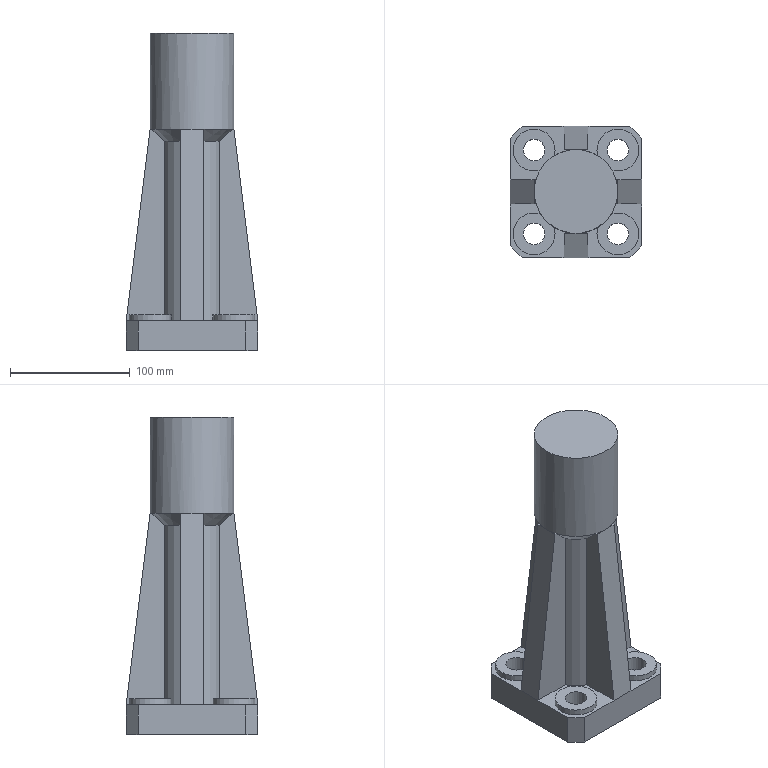Part | NX | features solid 2 | 1 solid | 55 faces | box 110 x 110 x 265 mm | volume 1177803 mm3 | plane 38 | cylinder 13 | cone 4 | commonest cylinder face diameters 18 x4 35 x4 50 x4 70 x1
STEP:
#1=CARTESIAN_POINT('',(935.,-402.087,-260.));
#2=VERTEX_POINT('',#1);
#3=CARTESIAN_POINT('',(935.,-402.087,-110.));
#4=VERTEX_POINT('',#3);
#5=CARTESIAN_POINT('',(935.,-402.087,-80.));
#6=DIRECTION('',(0.,0.,-1.));
#7=VECTOR('',#6,1000.);
#8=LINE('',#5,#7);
#9=EDGE_CURVE('',#2,#4,#8,.F.);
#10=ORIENTED_EDGE('',*,*,#9,.F.);
#11=CARTESIAN_POINT('',(922.087,-415.,-260.));
#12=VERTEX_POINT('',#11);
#13=CARTESIAN_POINT('',(945.,-425.,-260.));
#14=DIRECTION('',(0.,0.,1.));
#15=DIRECTION('',(1.,0.,0.));
#16=AXIS2_PLACEMENT_3D('',#13,#14,#15);
#17=CIRCLE('',#16,25.);
#18=EDGE_CURVE('',#12,#2,#17,.F.);
#19=ORIENTED_EDGE('',*,*,#18,.F.);
#20=CARTESIAN_POINT('',(922.087,-415.,-110.));
#21=VERTEX_POINT('',#20);
#22=CARTESIAN_POINT('',(922.087,-415.,-80.));
#23=DIRECTION('',(0.,0.,-1.));
#24=VECTOR('',#23,1000.);
#25=LINE('',#22,#24);
#26=EDGE_CURVE('',#12,#21,#25,.F.);
#27=ORIENTED_EDGE('',*,*,#26,.T.);
#28=CARTESIAN_POINT('',(945.,-425.,-110.));
#29=DIRECTION('',(0.,0.,1.));
#30=DIRECTION('',(1.,0.,0.));
#31=AXIS2_PLACEMENT_3D('',#28,#29,#30);
#32=CIRCLE('',#31,25.);
#33=EDGE_CURVE('',#21,#4,#32,.F.);
#34=ORIENTED_EDGE('',*,*,#33,.T.);
#35=EDGE_LOOP('',(#10,#19,#27,#34));
#36=FACE_BOUND('',#35,.T.);
#37=CARTESIAN_POINT('',(945.,-425.,-80.));
#38=DIRECTION('',(0.,0.,-1.));
#39=DIRECTION('',(-1.,0.,0.));
#40=AXIS2_PLACEMENT_3D('',#37,#38,#39);
#41=CYLINDRICAL_SURFACE('',#40,25.);
#42=ADVANCED_FACE('',(#36),#41,.T.);
#43=CARTESIAN_POINT('',(935.,-391.459,-100.));
#44=VERTEX_POINT('',#43);
#45=CARTESIAN_POINT('',(935.,-391.459,-100.));
#46=CARTESIAN_POINT('',(935.,-394.971,-103.366));
#47=CARTESIAN_POINT('',(935.,-398.501,-106.713));
#48=CARTESIAN_POINT('',(935.,-402.087,-110.));
#49=B_SPLINE_CURVE_WITH_KNOTS('',3,(#45,#46,#47,#48),.UNSPECIFIED.,.F.,.F.,(4,4),(0.01718,0.03177),.UNSPECIFIED.);
#50=EDGE_CURVE('',#4,#44,#49,.F.);
#51=ORIENTED_EDGE('',*,*,#50,.F.);
#52=ORIENTED_EDGE('',*,*,#33,.F.);
#53=CARTESIAN_POINT('',(911.459,-415.,-100.));
#54=VERTEX_POINT('',#53);
#55=CARTESIAN_POINT('',(911.459,-415.,-100.));
#56=CARTESIAN_POINT('',(914.971,-415.,-103.366));
#57=CARTESIAN_POINT('',(918.501,-415.,-106.713));
#58=CARTESIAN_POINT('',(922.087,-415.,-110.));
#59=B_SPLINE_CURVE_WITH_KNOTS('',3,(#55,#56,#57,#58),.UNSPECIFIED.,.F.,.F.,(4,4),(0.02378,0.03837),.UNSPECIFIED.);
#60=EDGE_CURVE('',#21,#54,#59,.F.);
#61=ORIENTED_EDGE('',*,*,#60,.T.);
#62=CARTESIAN_POINT('',(945.,-425.,-100.));
#63=DIRECTION('',(0.,0.,1.));
#64=DIRECTION('',(1.,0.,0.));
#65=AXIS2_PLACEMENT_3D('',#62,#63,#64);
#66=CIRCLE('',#65,35.);
#67=EDGE_CURVE('',#44,#54,#66,.T.);
#68=ORIENTED_EDGE('',*,*,#67,.F.);
#69=EDGE_LOOP('',(#51,#52,#61,#68));
#70=FACE_BOUND('',#69,.T.);
#71=CARTESIAN_POINT('',(945.,-425.,-100.));
#72=DIRECTION('',(0.,0.,1.));
#73=DIRECTION('',(1.,0.,0.));
#74=AXIS2_PLACEMENT_3D('',#71,#72,#73);
#75=CONICAL_SURFACE('',#74,35.,0.7854);
#76=ADVANCED_FACE('',(#70),#75,.T.);
#77=CARTESIAN_POINT('',(927.5,-390.,-260.));
#78=VERTEX_POINT('',#77);
#79=CARTESIAN_POINT('',(910.,-390.,-260.));
#80=DIRECTION('',(0.,0.,1.));
#81=DIRECTION('',(1.,0.,0.));
#82=AXIS2_PLACEMENT_3D('',#79,#80,#81);
#83=CIRCLE('',#82,17.5);
#84=EDGE_CURVE('',#78,#78,#83,.T.);
#85=ORIENTED_EDGE('',*,*,#84,.F.);
#86=EDGE_LOOP('',(#85));
#87=FACE_BOUND('',#86,.T.);
#88=CARTESIAN_POINT('',(900.,-370.,-260.));
#89=VERTEX_POINT('',#88);
#90=CARTESIAN_POINT('',(935.,-370.,-260.));
#91=VERTEX_POINT('',#90);
#92=CARTESIAN_POINT('',(890.,-370.,-260.));
#93=DIRECTION('',(1.,0.,0.));
#94=VECTOR('',#93,1000.);
#95=LINE('',#92,#94);
#96=EDGE_CURVE('',#89,#91,#95,.T.);
#97=ORIENTED_EDGE('',*,*,#96,.F.);
#98=CARTESIAN_POINT('',(890.,-380.,-260.));
#99=VERTEX_POINT('',#98);
#100=CARTESIAN_POINT('',(867.5,-402.5,-260.));
#101=DIRECTION('',(-0.7071,-0.7071,0.));
#102=VECTOR('',#101,1000.);
#103=LINE('',#100,#102);
#104=EDGE_CURVE('',#89,#99,#103,.T.);
#105=ORIENTED_EDGE('',*,*,#104,.T.);
#106=CARTESIAN_POINT('',(890.,-415.,-260.));
#107=VERTEX_POINT('',#106);
#108=CARTESIAN_POINT('',(890.,-425.,-260.));
#109=DIRECTION('',(0.,-1.,0.));
#110=VECTOR('',#109,1000.);
#111=LINE('',#108,#110);
#112=EDGE_CURVE('',#107,#99,#111,.F.);
#113=ORIENTED_EDGE('',*,*,#112,.F.);
#114=CARTESIAN_POINT('',(890.,-415.,-260.));
#115=DIRECTION('',(-1.,0.,0.));
#116=VECTOR('',#115,1000.);
#117=LINE('',#114,#116);
#118=EDGE_CURVE('',#12,#107,#117,.T.);
#119=ORIENTED_EDGE('',*,*,#118,.F.);
#120=ORIENTED_EDGE('',*,*,#18,.T.);
#121=CARTESIAN_POINT('',(935.,-425.,-260.));
#122=DIRECTION('',(0.,1.,0.));
#123=VECTOR('',#122,1000.);
#124=LINE('',#121,#123);
#125=EDGE_CURVE('',#2,#91,#124,.T.);
#126=ORIENTED_EDGE('',*,*,#125,.T.);
#127=EDGE_LOOP('',(#97,#105,#113,#119,#120,#126));
#128=FACE_BOUND('',#127,.T.);
#129=CARTESIAN_POINT('',(890.,-425.,-260.));
#130=DIRECTION('',(0.,0.,1.));
#131=DIRECTION('',(1.,0.,0.));
#132=AXIS2_PLACEMENT_3D('',#129,#130,#131);
#133=PLANE('',#132);
#134=ADVANCED_FACE('',(#87,#128),#133,.T.);
#135=CARTESIAN_POINT('',(922.087,-435.,-260.));
#136=VERTEX_POINT('',#135);
#137=CARTESIAN_POINT('',(922.087,-435.,-110.));
#138=VERTEX_POINT('',#137);
#139=CARTESIAN_POINT('',(922.087,-435.,-80.));
#140=DIRECTION('',(0.,0.,-1.));
#141=VECTOR('',#140,1000.);
#142=LINE('',#139,#141);
#143=EDGE_CURVE('',#136,#138,#142,.F.);
#144=ORIENTED_EDGE('',*,*,#143,.F.);
#145=CARTESIAN_POINT('',(935.,-447.913,-260.));
#146=VERTEX_POINT('',#145);
#147=CARTESIAN_POINT('',(945.,-425.,-260.));
#148=DIRECTION('',(0.,0.,1.));
#149=DIRECTION('',(1.,0.,0.));
#150=AXIS2_PLACEMENT_3D('',#147,#148,#149);
#151=CIRCLE('',#150,25.);
#152=EDGE_CURVE('',#146,#136,#151,.F.);
#153=ORIENTED_EDGE('',*,*,#152,.F.);
#154=CARTESIAN_POINT('',(935.,-447.913,-110.));
#155=VERTEX_POINT('',#154);
#156=CARTESIAN_POINT('',(935.,-447.913,-80.));
#157=DIRECTION('',(0.,0.,-1.));
#158=VECTOR('',#157,1000.);
#159=LINE('',#156,#158);
#160=EDGE_CURVE('',#146,#155,#159,.F.);
#161=ORIENTED_EDGE('',*,*,#160,.T.);
#162=CARTESIAN_POINT('',(945.,-425.,-110.));
#163=DIRECTION('',(0.,0.,1.));
#164=DIRECTION('',(1.,0.,0.));
#165=AXIS2_PLACEMENT_3D('',#162,#163,#164);
#166=CIRCLE('',#165,25.);
#167=EDGE_CURVE('',#155,#138,#166,.F.);
#168=ORIENTED_EDGE('',*,*,#167,.T.);
#169=EDGE_LOOP('',(#144,#153,#161,#168));
#170=FACE_BOUND('',#169,.T.);
#171=CARTESIAN_POINT('',(945.,-425.,-80.));
#172=DIRECTION('',(0.,0.,-1.));
#173=DIRECTION('',(-1.,0.,0.));
#174=AXIS2_PLACEMENT_3D('',#171,#172,#173);
#175=CYLINDRICAL_SURFACE('',#174,25.);
#176=ADVANCED_FACE('',(#170),#175,.T.);
#177=CARTESIAN_POINT('',(911.459,-435.,-100.));
#178=VERTEX_POINT('',#177);
#179=CARTESIAN_POINT('',(911.459,-435.,-100.));
#180=CARTESIAN_POINT('',(914.971,-435.,-103.366));
#181=CARTESIAN_POINT('',(918.501,-435.,-106.713));
#182=CARTESIAN_POINT('',(922.087,-435.,-110.));
#183=B_SPLINE_CURVE_WITH_KNOTS('',3,(#179,#180,#181,#182),.UNSPECIFIED.,.F.,.F.,(4,4),(0.02378,0.03837),.UNSPECIFIED.);
#184=EDGE_CURVE('',#138,#178,#183,.F.);
#185=ORIENTED_EDGE('',*,*,#184,.F.);
#186=ORIENTED_EDGE('',*,*,#167,.F.);
#187=CARTESIAN_POINT('',(935.,-458.541,-100.));
#188=VERTEX_POINT('',#187);
#189=CARTESIAN_POINT('',(935.,-458.541,-100.));
#190=CARTESIAN_POINT('',(935.,-455.029,-103.366));
#191=CARTESIAN_POINT('',(935.,-451.499,-106.713));
#192=CARTESIAN_POINT('',(935.,-447.913,-110.));
#193=B_SPLINE_CURVE_WITH_KNOTS('',3,(#189,#190,#191,#192),.UNSPECIFIED.,.F.,.F.,(4,4),(0.02378,0.03837),.UNSPECIFIED.);
#194=EDGE_CURVE('',#155,#188,#193,.F.);
#195=ORIENTED_EDGE('',*,*,#194,.T.);
#196=CARTESIAN_POINT('',(945.,-425.,-100.));
#197=DIRECTION('',(0.,0.,1.));
#198=DIRECTION('',(1.,0.,0.));
#199=AXIS2_PLACEMENT_3D('',#196,#197,#198);
#200=CIRCLE('',#199,35.);
#201=EDGE_CURVE('',#178,#188,#200,.T.);
#202=ORIENTED_EDGE('',*,*,#201,.F.);
#203=EDGE_LOOP('',(#185,#186,#195,#202));
#204=FACE_BOUND('',#203,.T.);
#205=CARTESIAN_POINT('',(945.,-425.,-100.));
#206=DIRECTION('',(0.,0.,1.));
#207=DIRECTION('',(1.,0.,0.));
#208=AXIS2_PLACEMENT_3D('',#205,#206,#207);
#209=CONICAL_SURFACE('',#208,35.,0.7854);
#210=ADVANCED_FACE('',(#204),#209,.T.);
#211=CARTESIAN_POINT('',(927.5,-460.,-260.));
#212=VERTEX_POINT('',#211);
#213=CARTESIAN_POINT('',(910.,-460.,-260.));
#214=DIRECTION('',(0.,0.,1.));
#215=DIRECTION('',(1.,0.,0.));
#216=AXIS2_PLACEMENT_3D('',#213,#214,#215);
#217=CIRCLE('',#216,17.5);
#218=EDGE_CURVE('',#212,#212,#217,.T.);
#219=ORIENTED_EDGE('',*,*,#218,.F.);
#220=EDGE_LOOP('',(#219));
#221=FACE_BOUND('',#220,.T.);
#222=CARTESIAN_POINT('',(890.,-470.,-260.));
#223=VERTEX_POINT('',#222);
#224=CARTESIAN_POINT('',(890.,-435.,-260.));
#225=VERTEX_POINT('',#224);
#226=CARTESIAN_POINT('',(890.,-425.,-260.));
#227=DIRECTION('',(0.,-1.,0.));
#228=VECTOR('',#227,1000.);
#229=LINE('',#226,#228);
#230=EDGE_CURVE('',#223,#225,#229,.F.);
#231=ORIENTED_EDGE('',*,*,#230,.F.);
#232=CARTESIAN_POINT('',(900.,-480.,-260.));
#233=VERTEX_POINT('',#232);
#234=CARTESIAN_POINT('',(867.5,-447.5,-260.));
#235=DIRECTION('',(-0.7071,0.7071,0.));
#236=VECTOR('',#235,1000.);
#237=LINE('',#234,#236);
#238=EDGE_CURVE('',#223,#233,#237,.F.);
#239=ORIENTED_EDGE('',*,*,#238,.T.);
#240=CARTESIAN_POINT('',(935.,-480.,-260.));
#241=VERTEX_POINT('',#240);
#242=CARTESIAN_POINT('',(890.,-480.,-260.));
#243=DIRECTION('',(1.,0.,0.));
#244=VECTOR('',#243,1000.);
#245=LINE('',#242,#244);
#246=EDGE_CURVE('',#233,#241,#245,.T.);
#247=ORIENTED_EDGE('',*,*,#246,.T.);
#248=CARTESIAN_POINT('',(935.,-425.,-260.));
#249=DIRECTION('',(0.,-1.,0.));
#250=VECTOR('',#249,1000.);
#251=LINE('',#248,#250);
#252=EDGE_CURVE('',#146,#241,#251,.T.);
#253=ORIENTED_EDGE('',*,*,#252,.F.);
#254=ORIENTED_EDGE('',*,*,#152,.T.);
#255=CARTESIAN_POINT('',(890.,-435.,-260.));
#256=DIRECTION('',(-1.,0.,0.));
#257=VECTOR('',#256,1000.);
#258=LINE('',#255,#257);
#259=EDGE_CURVE('',#136,#225,#258,.T.);
#260=ORIENTED_EDGE('',*,*,#259,.T.);
#261=EDGE_LOOP('',(#231,#239,#247,#253,#254,#260));
#262=FACE_BOUND('',#261,.T.);
#263=CARTESIAN_POINT('',(890.,-425.,-260.));
#264=DIRECTION('',(0.,0.,1.));
#265=DIRECTION('',(1.,0.,0.));
#266=AXIS2_PLACEMENT_3D('',#263,#264,#265);
#267=PLANE('',#266);
#268=ADVANCED_FACE('',(#221,#262),#267,.T.);
#269=CARTESIAN_POINT('',(955.,-402.087,-260.));
#270=VERTEX_POINT('',#269);
#271=CARTESIAN_POINT('',(967.913,-415.,-260.));
#272=VERTEX_POINT('',#271);
#273=CARTESIAN_POINT('',(945.,-425.,-260.));
#274=DIRECTION('',(0.,0.,1.));
#275=DIRECTION('',(1.,0.,0.));
#276=AXIS2_PLACEMENT_3D('',#273,#274,#275);
#277=CIRCLE('',#276,25.);
#278=EDGE_CURVE('',#270,#272,#277,.F.);
#279=ORIENTED_EDGE('',*,*,#278,.F.);
#280=CARTESIAN_POINT('',(955.,-402.087,-110.));
#281=VERTEX_POINT('',#280);
#282=CARTESIAN_POINT('',(955.,-402.087,-80.));
#283=DIRECTION('',(0.,0.,-1.));
#284=VECTOR('',#283,1000.);
#285=LINE('',#282,#284);
#286=EDGE_CURVE('',#270,#281,#285,.F.);
#287=ORIENTED_EDGE('',*,*,#286,.T.);
#288=CARTESIAN_POINT('',(967.913,-415.,-110.));
#289=VERTEX_POINT('',#288);
#290=CARTESIAN_POINT('',(945.,-425.,-110.));
#291=DIRECTION('',(0.,0.,1.));
#292=DIRECTION('',(1.,0.,0.));
#293=AXIS2_PLACEMENT_3D('',#290,#291,#292);
#294=CIRCLE('',#293,25.);
#295=EDGE_CURVE('',#281,#289,#294,.F.);
#296=ORIENTED_EDGE('',*,*,#295,.T.);
#297=CARTESIAN_POINT('',(967.913,-415.,-80.));
#298=DIRECTION('',(0.,0.,-1.));
#299=VECTOR('',#298,1000.);
#300=LINE('',#297,#299);
#301=EDGE_CURVE('',#272,#289,#300,.F.);
#302=ORIENTED_EDGE('',*,*,#301,.F.);
#303=EDGE_LOOP('',(#279,#287,#296,#302));
#304=FACE_BOUND('',#303,.T.);
#305=CARTESIAN_POINT('',(945.,-425.,-80.));
#306=DIRECTION('',(0.,0.,-1.));
#307=DIRECTION('',(-1.,0.,0.));
#308=AXIS2_PLACEMENT_3D('',#305,#306,#307);
#309=CYLINDRICAL_SURFACE('',#308,25.);
#310=ADVANCED_FACE('',(#304),#309,.T.);
#311=ORIENTED_EDGE('',*,*,#295,.F.);
#312=CARTESIAN_POINT('',(955.,-391.459,-100.));
#313=VERTEX_POINT('',#312);
#314=CARTESIAN_POINT('',(955.,-391.459,-100.));
#315=CARTESIAN_POINT('',(955.,-394.971,-103.366));
#316=CARTESIAN_POINT('',(955.,-398.501,-106.713));
#317=CARTESIAN_POINT('',(955.,-402.087,-110.));
#318=B_SPLINE_CURVE_WITH_KNOTS('',3,(#314,#315,#316,#317),.UNSPECIFIED.,.F.,.F.,(4,4),(0.01718,0.03177),.UNSPECIFIED.);
#319=EDGE_CURVE('',#281,#313,#318,.F.);
#320=ORIENTED_EDGE('',*,*,#319,.T.);
#321=CARTESIAN_POINT('',(978.541,-415.,-100.));
#322=VERTEX_POINT('',#321);
#323=CARTESIAN_POINT('',(945.,-425.,-100.));
#324=DIRECTION('',(0.,0.,1.));
#325=DIRECTION('',(1.,0.,0.));
#326=AXIS2_PLACEMENT_3D('',#323,#324,#325);
#327=CIRCLE('',#326,35.);
#328=EDGE_CURVE('',#322,#313,#327,.T.);
#329=ORIENTED_EDGE('',*,*,#328,.F.);
#330=CARTESIAN_POINT('',(978.541,-415.,-100.));
#331=CARTESIAN_POINT('',(975.029,-415.,-103.366));
#332=CARTESIAN_POINT('',(971.499,-415.,-106.713));
#333=CARTESIAN_POINT('',(967.913,-415.,-110.));
#334=B_SPLINE_CURVE_WITH_KNOTS('',3,(#330,#331,#332,#333),.UNSPECIFIED.,.F.,.F.,(4,4),(0.01718,0.03177),.UNSPECIFIED.);
#335=EDGE_CURVE('',#289,#322,#334,.F.);
#336=ORIENTED_EDGE('',*,*,#335,.F.);
#337=EDGE_LOOP('',(#311,#320,#329,#336));
#338=FACE_BOUND('',#337,.T.);
#339=CARTESIAN_POINT('',(945.,-425.,-100.));
#340=DIRECTION('',(0.,0.,1.));
#341=DIRECTION('',(1.,0.,0.));
#342=AXIS2_PLACEMENT_3D('',#339,#340,#341);
#343=CONICAL_SURFACE('',#342,35.,0.7854);
#344=ADVANCED_FACE('',(#338),#343,.T.);
#345=CARTESIAN_POINT('',(997.5,-390.,-260.));
#346=VERTEX_POINT('',#345);
#347=CARTESIAN_POINT('',(980.,-390.,-260.));
#348=DIRECTION('',(0.,0.,1.));
#349=DIRECTION('',(1.,0.,0.));
#350=AXIS2_PLACEMENT_3D('',#347,#348,#349);
#351=CIRCLE('',#350,17.5);
#352=EDGE_CURVE('',#346,#346,#351,.T.);
#353=ORIENTED_EDGE('',*,*,#352,.F.);
#354=EDGE_LOOP('',(#353));
#355=FACE_BOUND('',#354,.T.);
#356=CARTESIAN_POINT('',(1000.,-415.,-260.));
#357=VERTEX_POINT('',#356);
#358=CARTESIAN_POINT('',(1000.,-380.,-260.));
#359=VERTEX_POINT('',#358);
#360=CARTESIAN_POINT('',(1000.,-425.,-260.));
#361=DIRECTION('',(0.,1.,0.));
#362=VECTOR('',#361,1000.);
#363=LINE('',#360,#362);
#364=EDGE_CURVE('',#357,#359,#363,.T.);
#365=ORIENTED_EDGE('',*,*,#364,.T.);
#366=CARTESIAN_POINT('',(990.,-370.,-260.));
#367=VERTEX_POINT('',#366);
#368=CARTESIAN_POINT('',(967.5,-347.5,-260.));
#369=DIRECTION('',(0.7071,-0.7071,0.));
#370=VECTOR('',#369,1000.);
#371=LINE('',#368,#370);
#372=EDGE_CURVE('',#359,#367,#371,.F.);
#373=ORIENTED_EDGE('',*,*,#372,.T.);
#374=CARTESIAN_POINT('',(955.,-370.,-260.));
#375=VERTEX_POINT('',#374);
#376=CARTESIAN_POINT('',(890.,-370.,-260.));
#377=DIRECTION('',(1.,0.,0.));
#378=VECTOR('',#377,1000.);
#379=LINE('',#376,#378);
#380=EDGE_CURVE('',#375,#367,#379,.T.);
#381=ORIENTED_EDGE('',*,*,#380,.F.);
#382=CARTESIAN_POINT('',(955.,-425.,-260.));
#383=DIRECTION('',(0.,1.,0.));
#384=VECTOR('',#383,1000.);
#385=LINE('',#382,#384);
#386=EDGE_CURVE('',#270,#375,#385,.T.);
#387=ORIENTED_EDGE('',*,*,#386,.F.);
#388=ORIENTED_EDGE('',*,*,#278,.T.);
#389=CARTESIAN_POINT('',(890.,-415.,-260.));
#390=DIRECTION('',(1.,0.,0.));
#391=VECTOR('',#390,1000.);
#392=LINE('',#389,#391);
#393=EDGE_CURVE('',#272,#357,#392,.T.);
#394=ORIENTED_EDGE('',*,*,#393,.T.);
#395=EDGE_LOOP('',(#365,#373,#381,#387,#388,#394));
#396=FACE_BOUND('',#395,.T.);
#397=CARTESIAN_POINT('',(890.,-425.,-260.));
#398=DIRECTION('',(0.,0.,1.));
#399=DIRECTION('',(1.,0.,0.));
#400=AXIS2_PLACEMENT_3D('',#397,#398,#399);
#401=PLANE('',#400);
#402=ADVANCED_FACE('',(#355,#396),#401,.T.);
#403=CARTESIAN_POINT('',(967.913,-435.,-260.));
#404=VERTEX_POINT('',#403);
#405=CARTESIAN_POINT('',(955.,-447.913,-260.));
#406=VERTEX_POINT('',#405);
#407=CARTESIAN_POINT('',(945.,-425.,-260.));
#408=DIRECTION('',(0.,0.,1.));
#409=DIRECTION('',(1.,0.,0.));
#410=AXIS2_PLACEMENT_3D('',#407,#408,#409);
#411=CIRCLE('',#410,25.);
#412=EDGE_CURVE('',#404,#406,#411,.F.);
#413=ORIENTED_EDGE('',*,*,#412,.F.);
#414=CARTESIAN_POINT('',(967.913,-435.,-110.));
#415=VERTEX_POINT('',#414);
#416=CARTESIAN_POINT('',(967.913,-435.,-80.));
#417=DIRECTION('',(0.,0.,-1.));
#418=VECTOR('',#417,1000.);
#419=LINE('',#416,#418);
#420=EDGE_CURVE('',#404,#415,#419,.F.);
#421=ORIENTED_EDGE('',*,*,#420,.T.);
#422=CARTESIAN_POINT('',(955.,-447.913,-110.));
#423=VERTEX_POINT('',#422);
#424=CARTESIAN_POINT('',(945.,-425.,-110.));
#425=DIRECTION('',(0.,0.,1.));
#426=DIRECTION('',(1.,0.,0.));
#427=AXIS2_PLACEMENT_3D('',#424,#425,#426);
#428=CIRCLE('',#427,25.);
#429=EDGE_CURVE('',#415,#423,#428,.F.);
#430=ORIENTED_EDGE('',*,*,#429,.T.);
#431=CARTESIAN_POINT('',(955.,-447.913,-80.));
#432=DIRECTION('',(0.,0.,-1.));
#433=VECTOR('',#432,1000.);
#434=LINE('',#431,#433);
#435=EDGE_CURVE('',#406,#423,#434,.F.);
#436=ORIENTED_EDGE('',*,*,#435,.F.);
#437=EDGE_LOOP('',(#413,#421,#430,#436));
#438=FACE_BOUND('',#437,.T.);
#439=CARTESIAN_POINT('',(945.,-425.,-80.));
#440=DIRECTION('',(0.,0.,-1.));
#441=DIRECTION('',(-1.,0.,0.));
#442=AXIS2_PLACEMENT_3D('',#439,#440,#441);
#443=CYLINDRICAL_SURFACE('',#442,25.);
#444=ADVANCED_FACE('',(#438),#443,.T.);
#445=ORIENTED_EDGE('',*,*,#429,.F.);
#446=CARTESIAN_POINT('',(978.541,-435.,-100.));
#447=VERTEX_POINT('',#446);
#448=CARTESIAN_POINT('',(978.541,-435.,-100.));
#449=CARTESIAN_POINT('',(975.029,-435.,-103.366));
#450=CARTESIAN_POINT('',(971.499,-435.,-106.713));
#451=CARTESIAN_POINT('',(967.913,-435.,-110.));
#452=B_SPLINE_CURVE_WITH_KNOTS('',3,(#448,#449,#450,#451),.UNSPECIFIED.,.F.,.F.,(4,4),(0.01718,0.03177),.UNSPECIFIED.);
#453=EDGE_CURVE('',#415,#447,#452,.F.);
#454=ORIENTED_EDGE('',*,*,#453,.T.);
#455=CARTESIAN_POINT('',(955.,-458.541,-100.));
#456=VERTEX_POINT('',#455);
#457=CARTESIAN_POINT('',(945.,-425.,-100.));
#458=DIRECTION('',(0.,0.,1.));
#459=DIRECTION('',(1.,0.,0.));
#460=AXIS2_PLACEMENT_3D('',#457,#458,#459);
#461=CIRCLE('',#460,35.);
#462=EDGE_CURVE('',#456,#447,#461,.T.);
#463=ORIENTED_EDGE('',*,*,#462,.F.);
#464=CARTESIAN_POINT('',(955.,-458.541,-100.));
#465=CARTESIAN_POINT('',(955.,-455.029,-103.366));
#466=CARTESIAN_POINT('',(955.,-451.499,-106.713));
#467=CARTESIAN_POINT('',(955.,-447.913,-110.));
#468=B_SPLINE_CURVE_WITH_KNOTS('',3,(#464,#465,#466,#467),.UNSPECIFIED.,.F.,.F.,(4,4),(0.02378,0.03837),.UNSPECIFIED.);
#469=EDGE_CURVE('',#423,#456,#468,.F.);
#470=ORIENTED_EDGE('',*,*,#469,.F.);
#471=EDGE_LOOP('',(#445,#454,#463,#470));
#472=FACE_BOUND('',#471,.T.);
#473=CARTESIAN_POINT('',(945.,-425.,-100.));
#474=DIRECTION('',(0.,0.,1.));
#475=DIRECTION('',(1.,0.,0.));
#476=AXIS2_PLACEMENT_3D('',#473,#474,#475);
#477=CONICAL_SURFACE('',#476,35.,0.7854);
#478=ADVANCED_FACE('',(#472),#477,.T.);
#479=CARTESIAN_POINT('',(997.5,-460.,-260.));
#480=VERTEX_POINT('',#479);
#481=CARTESIAN_POINT('',(980.,-460.,-260.));
#482=DIRECTION('',(0.,0.,1.));
#483=DIRECTION('',(1.,0.,0.));
#484=AXIS2_PLACEMENT_3D('',#481,#482,#483);
#485=CIRCLE('',#484,17.5);
#486=EDGE_CURVE('',#480,#480,#485,.T.);
#487=ORIENTED_EDGE('',*,*,#486,.F.);
#488=EDGE_LOOP('',(#487));
#489=FACE_BOUND('',#488,.T.);
#490=CARTESIAN_POINT('',(955.,-480.,-260.));
#491=VERTEX_POINT('',#490);
#492=CARTESIAN_POINT('',(990.,-480.,-260.));
#493=VERTEX_POINT('',#492);
#494=CARTESIAN_POINT('',(890.,-480.,-260.));
#495=DIRECTION('',(1.,0.,0.));
#496=VECTOR('',#495,1000.);
#497=LINE('',#494,#496);
#498=EDGE_CURVE('',#491,#493,#497,.T.);
#499=ORIENTED_EDGE('',*,*,#498,.T.);
#500=CARTESIAN_POINT('',(1000.,-470.,-260.));
#501=VERTEX_POINT('',#500);
#502=CARTESIAN_POINT('',(967.5,-502.5,-260.));
#503=DIRECTION('',(0.7071,0.7071,0.));
#504=VECTOR('',#503,1000.);
#505=LINE('',#502,#504);
#506=EDGE_CURVE('',#493,#501,#505,.T.);
#507=ORIENTED_EDGE('',*,*,#506,.T.);
#508=CARTESIAN_POINT('',(1000.,-435.,-260.));
#509=VERTEX_POINT('',#508);
#510=CARTESIAN_POINT('',(1000.,-425.,-260.));
#511=DIRECTION('',(0.,1.,0.));
#512=VECTOR('',#511,1000.);
#513=LINE('',#510,#512);
#514=EDGE_CURVE('',#501,#509,#513,.T.);
#515=ORIENTED_EDGE('',*,*,#514,.T.);
#516=CARTESIAN_POINT('',(890.,-435.,-260.));
#517=DIRECTION('',(1.,0.,0.));
#518=VECTOR('',#517,1000.);
#519=LINE('',#516,#518);
#520=EDGE_CURVE('',#404,#509,#519,.T.);
#521=ORIENTED_EDGE('',*,*,#520,.F.);
#522=ORIENTED_EDGE('',*,*,#412,.T.);
#523=CARTESIAN_POINT('',(955.,-425.,-260.));
#524=DIRECTION('',(0.,-1.,0.));
#525=VECTOR('',#524,1000.);
#526=LINE('',#523,#525);
#527=EDGE_CURVE('',#406,#491,#526,.T.);
#528=ORIENTED_EDGE('',*,*,#527,.T.);
#529=EDGE_LOOP('',(#499,#507,#515,#521,#522,#528));
#530=FACE_BOUND('',#529,.T.);
#531=CARTESIAN_POINT('',(890.,-425.,-260.));
#532=DIRECTION('',(0.,0.,1.));
#533=DIRECTION('',(1.,0.,0.));
#534=AXIS2_PLACEMENT_3D('',#531,#532,#533);
#535=PLANE('',#534);
#536=ADVANCED_FACE('',(#489,#530),#535,.T.);
#537=CARTESIAN_POINT('',(945.,-460.,-100.));
#538=VERTEX_POINT('',#537);
#539=CARTESIAN_POINT('',(945.,-425.,-100.));
#540=DIRECTION('',(0.,0.,1.));
#541=DIRECTION('',(1.,0.,0.));
#542=AXIS2_PLACEMENT_3D('',#539,#540,#541);
#543=CIRCLE('',#542,35.);
#544=EDGE_CURVE('',#188,#538,#543,.T.);
#545=ORIENTED_EDGE('',*,*,#544,.T.);
#546=CARTESIAN_POINT('',(945.,-425.,-100.));
#547=DIRECTION('',(0.,0.,1.));
#548=DIRECTION('',(1.,0.,0.));
#549=AXIS2_PLACEMENT_3D('',#546,#547,#548);
#550=CIRCLE('',#549,35.);
#551=EDGE_CURVE('',#538,#456,#550,.T.);
#552=ORIENTED_EDGE('',*,*,#551,.T.);
#553=ORIENTED_EDGE('',*,*,#462,.T.);
#554=CARTESIAN_POINT('',(980.,-425.,-100.));
#555=VERTEX_POINT('',#554);
#556=CARTESIAN_POINT('',(945.,-425.,-100.));
#557=DIRECTION('',(0.,0.,1.));
#558=DIRECTION('',(1.,0.,0.));
#559=AXIS2_PLACEMENT_3D('',#556,#557,#558);
#560=CIRCLE('',#559,35.);
#561=EDGE_CURVE('',#447,#555,#560,.T.);
#562=ORIENTED_EDGE('',*,*,#561,.T.);
#563=CARTESIAN_POINT('',(945.,-425.,-100.));
#564=DIRECTION('',(0.,0.,1.));
#565=DIRECTION('',(1.,0.,0.));
#566=AXIS2_PLACEMENT_3D('',#563,#564,#565);
#567=CIRCLE('',#566,35.);
#568=EDGE_CURVE('',#555,#322,#567,.T.);
#569=ORIENTED_EDGE('',*,*,#568,.T.);
#570=ORIENTED_EDGE('',*,*,#328,.T.);
#571=CARTESIAN_POINT('',(945.,-390.,-100.));
#572=VERTEX_POINT('',#571);
#573=CARTESIAN_POINT('',(945.,-425.,-100.));
#574=DIRECTION('',(0.,0.,1.));
#575=DIRECTION('',(1.,0.,0.));
#576=AXIS2_PLACEMENT_3D('',#573,#574,#575);
#577=CIRCLE('',#576,35.);
#578=EDGE_CURVE('',#313,#572,#577,.T.);
#579=ORIENTED_EDGE('',*,*,#578,.T.);
#580=CARTESIAN_POINT('',(945.,-425.,-100.));
#581=DIRECTION('',(0.,0.,1.));
#582=DIRECTION('',(1.,0.,0.));
#583=AXIS2_PLACEMENT_3D('',#580,#581,#582);
#584=CIRCLE('',#583,35.);
#585=EDGE_CURVE('',#572,#44,#584,.T.);
#586=ORIENTED_EDGE('',*,*,#585,.T.);
#587=ORIENTED_EDGE('',*,*,#67,.T.);
#588=CARTESIAN_POINT('',(910.,-425.,-100.));
#589=VERTEX_POINT('',#588);
#590=CARTESIAN_POINT('',(945.,-425.,-100.));
#591=DIRECTION('',(0.,0.,1.));
#592=DIRECTION('',(1.,0.,0.));
#593=AXIS2_PLACEMENT_3D('',#590,#591,#592);
#594=CIRCLE('',#593,35.);
#595=EDGE_CURVE('',#54,#589,#594,.T.);
#596=ORIENTED_EDGE('',*,*,#595,.T.);
#597=CARTESIAN_POINT('',(945.,-425.,-100.));
#598=DIRECTION('',(0.,0.,1.));
#599=DIRECTION('',(1.,0.,0.));
#600=AXIS2_PLACEMENT_3D('',#597,#598,#599);
#601=CIRCLE('',#600,35.);
#602=EDGE_CURVE('',#589,#178,#601,.T.);
#603=ORIENTED_EDGE('',*,*,#602,.T.);
#604=ORIENTED_EDGE('',*,*,#201,.T.);
#605=EDGE_LOOP('',(#545,#552,#553,#562,#569,#570,#579,#586,#587,#596,#603,#604));
#606=FACE_BOUND('',#605,.T.);
#607=CARTESIAN_POINT('',(980.,-425.,-20.));
#608=VERTEX_POINT('',#607);
#609=CARTESIAN_POINT('',(945.,-425.,-20.));
#610=DIRECTION('',(0.,0.,-1.));
#611=DIRECTION('',(1.,0.,0.));
#612=AXIS2_PLACEMENT_3D('',#609,#610,#611);
#613=CIRCLE('',#612,35.);
#614=EDGE_CURVE('',#608,#608,#613,.F.);
#615=ORIENTED_EDGE('',*,*,#614,.F.);
#616=EDGE_LOOP('',(#615));
#617=FACE_BOUND('',#616,.T.);
#618=CARTESIAN_POINT('',(945.,-425.,-140.));
#619=DIRECTION('',(0.,0.,1.));
#620=DIRECTION('',(1.,0.,0.));
#621=AXIS2_PLACEMENT_3D('',#618,#619,#620);
#622=CYLINDRICAL_SURFACE('',#621,35.);
#623=ADVANCED_FACE('',(#606,#617),#622,.T.);
#624=ORIENTED_EDGE('',*,*,#614,.T.);
#625=EDGE_LOOP('',(#624));
#626=FACE_BOUND('',#625,.T.);
#627=CARTESIAN_POINT('',(945.,-425.,-20.));
#628=DIRECTION('',(0.,0.,1.));
#629=DIRECTION('',(1.,0.,0.));
#630=AXIS2_PLACEMENT_3D('',#627,#628,#629);
#631=PLANE('',#630);
#632=ADVANCED_FACE('',(#626),#631,.T.);
#633=CARTESIAN_POINT('',(1000.,-470.,-285.));
#634=VERTEX_POINT('',#633);
#635=CARTESIAN_POINT('',(1000.,-380.,-285.));
#636=VERTEX_POINT('',#635);
#637=CARTESIAN_POINT('',(1000.,-425.,-285.));
#638=DIRECTION('',(0.,-1.,0.));
#639=VECTOR('',#638,1000.);
#640=LINE('',#637,#639);
#641=EDGE_CURVE('',#634,#636,#640,.F.);
#642=ORIENTED_EDGE('',*,*,#641,.T.);
#643=CARTESIAN_POINT('',(1000.,-380.,-265.));
#644=DIRECTION('',(0.,0.,1.));
#645=VECTOR('',#644,1000.);
#646=LINE('',#643,#645);
#647=EDGE_CURVE('',#636,#359,#646,.T.);
#648=ORIENTED_EDGE('',*,*,#647,.T.);
#649=ORIENTED_EDGE('',*,*,#364,.F.);
#650=CARTESIAN_POINT('',(1000.,-425.,-260.));
#651=DIRECTION('',(0.,1.,0.));
#652=VECTOR('',#651,1000.);
#653=LINE('',#650,#652);
#654=EDGE_CURVE('',#357,#509,#653,.F.);
#655=ORIENTED_EDGE('',*,*,#654,.T.);
#656=ORIENTED_EDGE('',*,*,#514,.F.);
#657=CARTESIAN_POINT('',(1000.,-470.,-295.));
#658=DIRECTION('',(0.,0.,-1.));
#659=VECTOR('',#658,1000.);
#660=LINE('',#657,#659);
#661=EDGE_CURVE('',#501,#634,#660,.T.);
#662=ORIENTED_EDGE('',*,*,#661,.T.);
#663=EDGE_LOOP('',(#642,#648,#649,#655,#656,#662));
#664=FACE_BOUND('',#663,.T.);
#665=CARTESIAN_POINT('',(1000.,-425.,-265.));
#666=DIRECTION('',(1.,0.,0.));
#667=DIRECTION('',(0.,0.,-1.));
#668=AXIS2_PLACEMENT_3D('',#665,#666,#667);
#669=PLANE('',#668);
#670=ADVANCED_FACE('',(#664),#669,.T.);
#671=CARTESIAN_POINT('',(919.,-390.,-285.));
#672=VERTEX_POINT('',#671);
#673=CARTESIAN_POINT('',(910.,-390.,-285.));
#674=DIRECTION('',(0.,0.,1.));
#675=DIRECTION('',(1.,0.,0.));
#676=AXIS2_PLACEMENT_3D('',#673,#674,#675);
#677=CIRCLE('',#676,9.);
#678=EDGE_CURVE('',#672,#672,#677,.F.);
#679=ORIENTED_EDGE('',*,*,#678,.F.);
#680=EDGE_LOOP('',(#679));
#681=FACE_BOUND('',#680,.T.);
#682=CARTESIAN_POINT('',(989.,-390.,-285.));
#683=VERTEX_POINT('',#682);
#684=CARTESIAN_POINT('',(980.,-390.,-285.));
#685=DIRECTION('',(0.,0.,1.));
#686=DIRECTION('',(1.,0.,0.));
#687=AXIS2_PLACEMENT_3D('',#684,#685,#686);
#688=CIRCLE('',#687,9.);
#689=EDGE_CURVE('',#683,#683,#688,.F.);
#690=ORIENTED_EDGE('',*,*,#689,.F.);
#691=EDGE_LOOP('',(#690));
#692=FACE_BOUND('',#691,.T.);
#693=CARTESIAN_POINT('',(919.,-460.,-285.));
#694=VERTEX_POINT('',#693);
#695=CARTESIAN_POINT('',(910.,-460.,-285.));
#696=DIRECTION('',(0.,0.,1.));
#697=DIRECTION('',(1.,0.,0.));
#698=AXIS2_PLACEMENT_3D('',#695,#696,#697);
#699=CIRCLE('',#698,9.);
#700=EDGE_CURVE('',#694,#694,#699,.F.);
#701=ORIENTED_EDGE('',*,*,#700,.F.);
#702=EDGE_LOOP('',(#701));
#703=FACE_BOUND('',#702,.T.);
#704=CARTESIAN_POINT('',(989.,-460.,-285.));
#705=VERTEX_POINT('',#704);
#706=CARTESIAN_POINT('',(980.,-460.,-285.));
#707=DIRECTION('',(0.,0.,1.));
#708=DIRECTION('',(1.,0.,0.));
#709=AXIS2_PLACEMENT_3D('',#706,#707,#708);
#710=CIRCLE('',#709,9.);
#711=EDGE_CURVE('',#705,#705,#710,.F.);
#712=ORIENTED_EDGE('',*,*,#711,.F.);
#713=EDGE_LOOP('',(#712));
#714=FACE_BOUND('',#713,.T.);
#715=CARTESIAN_POINT('',(890.,-470.,-285.));
#716=VERTEX_POINT('',#715);
#717=CARTESIAN_POINT('',(890.,-380.,-285.));
#718=VERTEX_POINT('',#717);
#719=CARTESIAN_POINT('',(890.,-425.,-285.));
#720=DIRECTION('',(0.,1.,0.));
#721=VECTOR('',#720,1000.);
#722=LINE('',#719,#721);
#723=EDGE_CURVE('',#716,#718,#722,.T.);
#724=ORIENTED_EDGE('',*,*,#723,.T.);
#725=CARTESIAN_POINT('',(900.,-370.,-285.));
#726=VERTEX_POINT('',#725);
#727=CARTESIAN_POINT('',(867.5,-402.5,-285.));
#728=DIRECTION('',(-0.7071,-0.7071,0.));
#729=VECTOR('',#728,1000.);
#730=LINE('',#727,#729);
#731=EDGE_CURVE('',#718,#726,#730,.F.);
#732=ORIENTED_EDGE('',*,*,#731,.T.);
#733=CARTESIAN_POINT('',(990.,-370.,-285.));
#734=VERTEX_POINT('',#733);
#735=CARTESIAN_POINT('',(890.,-370.,-285.));
#736=DIRECTION('',(-1.,0.,0.));
#737=VECTOR('',#736,1000.);
#738=LINE('',#735,#737);
#739=EDGE_CURVE('',#726,#734,#738,.F.);
#740=ORIENTED_EDGE('',*,*,#739,.T.);
#741=CARTESIAN_POINT('',(967.5,-347.5,-285.));
#742=DIRECTION('',(0.7071,-0.7071,0.));
#743=VECTOR('',#742,1000.);
#744=LINE('',#741,#743);
#745=EDGE_CURVE('',#734,#636,#744,.T.);
#746=ORIENTED_EDGE('',*,*,#745,.T.);
#747=ORIENTED_EDGE('',*,*,#641,.F.);
#748=CARTESIAN_POINT('',(990.,-480.,-285.));
#749=VERTEX_POINT('',#748);
#750=CARTESIAN_POINT('',(967.5,-502.5,-285.));
#751=DIRECTION('',(0.7071,0.7071,0.));
#752=VECTOR('',#751,1000.);
#753=LINE('',#750,#752);
#754=EDGE_CURVE('',#634,#749,#753,.F.);
#755=ORIENTED_EDGE('',*,*,#754,.T.);
#756=CARTESIAN_POINT('',(900.,-480.,-285.));
#757=VERTEX_POINT('',#756);
#758=CARTESIAN_POINT('',(890.,-480.,-285.));
#759=DIRECTION('',(-1.,0.,0.));
#760=VECTOR('',#759,1000.);
#761=LINE('',#758,#760);
#762=EDGE_CURVE('',#757,#749,#761,.F.);
#763=ORIENTED_EDGE('',*,*,#762,.F.);
#764=CARTESIAN_POINT('',(867.5,-447.5,-285.));
#765=DIRECTION('',(-0.7071,0.7071,0.));
#766=VECTOR('',#765,1000.);
#767=LINE('',#764,#766);
#768=EDGE_CURVE('',#757,#716,#767,.T.);
#769=ORIENTED_EDGE('',*,*,#768,.T.);
#770=EDGE_LOOP('',(#724,#732,#740,#746,#747,#755,#763,#769));
#771=FACE_BOUND('',#770,.T.);
#772=CARTESIAN_POINT('',(890.,-425.,-285.));
#773=DIRECTION('',(0.,0.,1.));
#774=DIRECTION('',(1.,0.,0.));
#775=AXIS2_PLACEMENT_3D('',#772,#773,#774);
#776=PLANE('',#775);
#777=ADVANCED_FACE('',(#681,#692,#703,#714,#771),#776,.F.);
#778=ORIENTED_EDGE('',*,*,#112,.T.);
#779=CARTESIAN_POINT('',(890.,-380.,-265.));
#780=DIRECTION('',(0.,0.,1.));
#781=VECTOR('',#780,1000.);
#782=LINE('',#779,#781);
#783=EDGE_CURVE('',#99,#718,#782,.F.);
#784=ORIENTED_EDGE('',*,*,#783,.T.);
#785=ORIENTED_EDGE('',*,*,#723,.F.);
#786=CARTESIAN_POINT('',(890.,-470.,-270.));
#787=DIRECTION('',(0.,0.,-1.));
#788=VECTOR('',#787,1000.);
#789=LINE('',#786,#788);
#790=EDGE_CURVE('',#716,#223,#789,.F.);
#791=ORIENTED_EDGE('',*,*,#790,.T.);
#792=ORIENTED_EDGE('',*,*,#230,.T.);
#793=CARTESIAN_POINT('',(890.,-425.,-260.));
#794=DIRECTION('',(0.,-1.,0.));
#795=VECTOR('',#794,1000.);
#796=LINE('',#793,#795);
#797=EDGE_CURVE('',#225,#107,#796,.F.);
#798=ORIENTED_EDGE('',*,*,#797,.T.);
#799=EDGE_LOOP('',(#778,#784,#785,#791,#792,#798));
#800=FACE_BOUND('',#799,.T.);
#801=CARTESIAN_POINT('',(890.,-425.,-265.));
#802=DIRECTION('',(1.,0.,0.));
#803=DIRECTION('',(0.,0.,-1.));
#804=AXIS2_PLACEMENT_3D('',#801,#802,#803);
#805=PLANE('',#804);
#806=ADVANCED_FACE('',(#800),#805,.F.);
#807=ORIENTED_EDGE('',*,*,#739,.F.);
#808=CARTESIAN_POINT('',(900.,-370.,-265.));
#809=DIRECTION('',(0.,0.,1.));
#810=VECTOR('',#809,1000.);
#811=LINE('',#808,#810);
#812=EDGE_CURVE('',#726,#89,#811,.T.);
#813=ORIENTED_EDGE('',*,*,#812,.T.);
#814=ORIENTED_EDGE('',*,*,#96,.T.);
#815=CARTESIAN_POINT('',(945.,-370.,-260.));
#816=DIRECTION('',(-1.,0.,0.));
#817=VECTOR('',#816,1000.);
#818=LINE('',#815,#817);
#819=EDGE_CURVE('',#91,#375,#818,.F.);
#820=ORIENTED_EDGE('',*,*,#819,.T.);
#821=ORIENTED_EDGE('',*,*,#380,.T.);
#822=CARTESIAN_POINT('',(990.,-370.,-265.));
#823=DIRECTION('',(0.,0.,-1.));
#824=VECTOR('',#823,1000.);
#825=LINE('',#822,#824);
#826=EDGE_CURVE('',#367,#734,#825,.T.);
#827=ORIENTED_EDGE('',*,*,#826,.T.);
#828=EDGE_LOOP('',(#807,#813,#814,#820,#821,#827));
#829=FACE_BOUND('',#828,.T.);
#830=CARTESIAN_POINT('',(890.,-370.,-265.));
#831=DIRECTION('',(0.,1.,0.));
#832=DIRECTION('',(0.,0.,1.));
#833=AXIS2_PLACEMENT_3D('',#830,#831,#832);
#834=PLANE('',#833);
#835=ADVANCED_FACE('',(#829),#834,.T.);
#836=ORIENTED_EDGE('',*,*,#246,.F.);
#837=CARTESIAN_POINT('',(900.,-480.,-295.));
#838=DIRECTION('',(0.,0.,-1.));
#839=VECTOR('',#838,1000.);
#840=LINE('',#837,#839);
#841=EDGE_CURVE('',#233,#757,#840,.T.);
#842=ORIENTED_EDGE('',*,*,#841,.T.);
#843=ORIENTED_EDGE('',*,*,#762,.T.);
#844=CARTESIAN_POINT('',(990.,-480.,-270.));
#845=DIRECTION('',(0.,0.,1.));
#846=VECTOR('',#845,1000.);
#847=LINE('',#844,#846);
#848=EDGE_CURVE('',#749,#493,#847,.T.);
#849=ORIENTED_EDGE('',*,*,#848,.T.);
#850=ORIENTED_EDGE('',*,*,#498,.F.);
#851=CARTESIAN_POINT('',(945.,-480.,-260.));
#852=DIRECTION('',(1.,0.,0.));
#853=VECTOR('',#852,1000.);
#854=LINE('',#851,#853);
#855=EDGE_CURVE('',#491,#241,#854,.F.);
#856=ORIENTED_EDGE('',*,*,#855,.T.);
#857=EDGE_LOOP('',(#836,#842,#843,#849,#850,#856));
#858=FACE_BOUND('',#857,.T.);
#859=CARTESIAN_POINT('',(890.,-480.,-265.));
#860=DIRECTION('',(0.,1.,0.));
#861=DIRECTION('',(0.,0.,1.));
#862=AXIS2_PLACEMENT_3D('',#859,#860,#861);
#863=PLANE('',#862);
#864=ADVANCED_FACE('',(#858),#863,.F.);
#865=CARTESIAN_POINT('',(955.,-460.,-100.));
#866=VERTEX_POINT('',#865);
#867=CARTESIAN_POINT('',(955.,-450.,-100.));
#868=DIRECTION('',(0.,-1.,0.));
#869=VECTOR('',#868,1000.);
#870=LINE('',#867,#869);
#871=EDGE_CURVE('',#456,#866,#870,.T.);
#872=ORIENTED_EDGE('',*,*,#871,.F.);
#873=ORIENTED_EDGE('',*,*,#551,.F.);
#874=CARTESIAN_POINT('',(945.,-460.,-100.));
#875=DIRECTION('',(1.,0.,0.));
#876=VECTOR('',#875,1000.);
#877=LINE('',#874,#876);
#878=EDGE_CURVE('',#538,#866,#877,.T.);
#879=ORIENTED_EDGE('',*,*,#878,.T.);
#880=EDGE_LOOP('',(#872,#873,#879));
#881=FACE_BOUND('',#880,.T.);
#882=CARTESIAN_POINT('',(945.,-450.,-100.));
#883=DIRECTION('',(0.,0.,-1.));
#884=DIRECTION('',(0.,-1.,0.));
#885=AXIS2_PLACEMENT_3D('',#882,#883,#884);
#886=PLANE('',#885);
#887=ADVANCED_FACE('',(#881),#886,.F.);
#888=CARTESIAN_POINT('',(935.,-460.,-100.));
#889=VERTEX_POINT('',#888);
#890=CARTESIAN_POINT('',(945.,-460.,-100.));
#891=DIRECTION('',(1.,0.,0.));
#892=VECTOR('',#891,1000.);
#893=LINE('',#890,#892);
#894=EDGE_CURVE('',#889,#538,#893,.T.);
#895=ORIENTED_EDGE('',*,*,#894,.T.);
#896=ORIENTED_EDGE('',*,*,#544,.F.);
#897=CARTESIAN_POINT('',(935.,-450.,-100.));
#898=DIRECTION('',(0.,-1.,0.));
#899=VECTOR('',#898,1000.);
#900=LINE('',#897,#899);
#901=EDGE_CURVE('',#188,#889,#900,.T.);
#902=ORIENTED_EDGE('',*,*,#901,.T.);
#903=EDGE_LOOP('',(#895,#896,#902));
#904=FACE_BOUND('',#903,.T.);
#905=CARTESIAN_POINT('',(945.,-450.,-100.));
#906=DIRECTION('',(0.,0.,-1.));
#907=DIRECTION('',(0.,-1.,0.));
#908=AXIS2_PLACEMENT_3D('',#905,#906,#907);
#909=PLANE('',#908);
#910=ADVANCED_FACE('',(#904),#909,.F.);
#911=ORIENTED_EDGE('',*,*,#527,.F.);
#912=ORIENTED_EDGE('',*,*,#435,.T.);
#913=ORIENTED_EDGE('',*,*,#469,.T.);
#914=ORIENTED_EDGE('',*,*,#871,.T.);
#915=CARTESIAN_POINT('',(955.,-460.,-100.));
#916=DIRECTION('',(0.,-0.124,-0.9923));
#917=VECTOR('',#916,1000.);
#918=LINE('',#915,#917);
#919=EDGE_CURVE('',#866,#491,#918,.T.);
#920=ORIENTED_EDGE('',*,*,#919,.T.);
#921=EDGE_LOOP('',(#911,#912,#913,#914,#920));
#922=FACE_BOUND('',#921,.T.);
#923=CARTESIAN_POINT('',(955.,-450.,-270.));
#924=DIRECTION('',(-1.,0.,0.));
#925=DIRECTION('',(0.,0.,-1.));
#926=AXIS2_PLACEMENT_3D('',#923,#924,#925);
#927=PLANE('',#926);
#928=ADVANCED_FACE('',(#922),#927,.F.);
#929=ORIENTED_EDGE('',*,*,#160,.F.);
#930=ORIENTED_EDGE('',*,*,#252,.T.);
#931=CARTESIAN_POINT('',(935.,-480.769,-266.154));
#932=DIRECTION('',(0.,0.124,0.9923));
#933=VECTOR('',#932,1000.);
#934=LINE('',#931,#933);
#935=EDGE_CURVE('',#241,#889,#934,.T.);
#936=ORIENTED_EDGE('',*,*,#935,.T.);
#937=ORIENTED_EDGE('',*,*,#901,.F.);
#938=ORIENTED_EDGE('',*,*,#194,.F.);
#939=EDGE_LOOP('',(#929,#930,#936,#937,#938));
#940=FACE_BOUND('',#939,.T.);
#941=CARTESIAN_POINT('',(935.,-450.,-270.));
#942=DIRECTION('',(-1.,0.,0.));
#943=DIRECTION('',(0.,0.,-1.));
#944=AXIS2_PLACEMENT_3D('',#941,#942,#943);
#945=PLANE('',#944);
#946=ADVANCED_FACE('',(#940),#945,.T.);
#947=ORIENTED_EDGE('',*,*,#935,.F.);
#948=ORIENTED_EDGE('',*,*,#855,.F.);
#949=ORIENTED_EDGE('',*,*,#919,.F.);
#950=ORIENTED_EDGE('',*,*,#878,.F.);
#951=ORIENTED_EDGE('',*,*,#894,.F.);
#952=EDGE_LOOP('',(#947,#948,#949,#950,#951));
#953=FACE_BOUND('',#952,.T.);
#954=CARTESIAN_POINT('',(945.,-460.,-100.));
#955=DIRECTION('',(0.,-0.9923,0.124));
#956=DIRECTION('',(0.,-0.124,-0.9923));
#957=AXIS2_PLACEMENT_3D('',#954,#955,#956);
#958=PLANE('',#957);
#959=ADVANCED_FACE('',(#953),#958,.T.);
#960=ORIENTED_EDGE('',*,*,#393,.F.);
#961=ORIENTED_EDGE('',*,*,#301,.T.);
#962=ORIENTED_EDGE('',*,*,#335,.T.);
#963=CARTESIAN_POINT('',(980.,-415.,-100.));
#964=VERTEX_POINT('',#963);
#965=CARTESIAN_POINT('',(970.,-415.,-100.));
#966=DIRECTION('',(1.,0.,0.));
#967=VECTOR('',#966,1000.);
#968=LINE('',#965,#967);
#969=EDGE_CURVE('',#322,#964,#968,.T.);
#970=ORIENTED_EDGE('',*,*,#969,.T.);
#971=CARTESIAN_POINT('',(980.,-415.,-100.));
#972=DIRECTION('',(0.124,0.,-0.9923));
#973=VECTOR('',#972,1000.);
#974=LINE('',#971,#973);
#975=EDGE_CURVE('',#964,#357,#974,.T.);
#976=ORIENTED_EDGE('',*,*,#975,.T.);
#977=EDGE_LOOP('',(#960,#961,#962,#970,#976));
#978=FACE_BOUND('',#977,.T.);
#979=CARTESIAN_POINT('',(970.,-415.,-270.));
#980=DIRECTION('',(0.,-1.,0.));
#981=DIRECTION('',(0.,0.,-1.));
#982=AXIS2_PLACEMENT_3D('',#979,#980,#981);
#983=PLANE('',#982);
#984=ADVANCED_FACE('',(#978),#983,.F.);
#985=ORIENTED_EDGE('',*,*,#420,.F.);
#986=ORIENTED_EDGE('',*,*,#520,.T.);
#987=CARTESIAN_POINT('',(980.,-435.,-100.));
#988=VERTEX_POINT('',#987);
#989=CARTESIAN_POINT('',(1000.769,-435.,-266.154));
#990=DIRECTION('',(-0.124,0.,0.9923));
#991=VECTOR('',#990,1000.);
#992=LINE('',#989,#991);
#993=EDGE_CURVE('',#509,#988,#992,.T.);
#994=ORIENTED_EDGE('',*,*,#993,.T.);
#995=CARTESIAN_POINT('',(970.,-435.,-100.));
#996=DIRECTION('',(1.,0.,0.));
#997=VECTOR('',#996,1000.);
#998=LINE('',#995,#997);
#999=EDGE_CURVE('',#447,#988,#998,.T.);
#1000=ORIENTED_EDGE('',*,*,#999,.F.);
#1001=ORIENTED_EDGE('',*,*,#453,.F.);
#1002=EDGE_LOOP('',(#985,#986,#994,#1000,#1001));
#1003=FACE_BOUND('',#1002,.T.);
#1004=CARTESIAN_POINT('',(970.,-435.,-270.));
#1005=DIRECTION('',(0.,-1.,0.));
#1006=DIRECTION('',(0.,0.,-1.));
#1007=AXIS2_PLACEMENT_3D('',#1004,#1005,#1006);
#1008=PLANE('',#1007);
#1009=ADVANCED_FACE('',(#1003),#1008,.T.);
#1010=ORIENTED_EDGE('',*,*,#561,.F.);
#1011=ORIENTED_EDGE('',*,*,#999,.T.);
#1012=CARTESIAN_POINT('',(980.,-425.,-100.));
#1013=DIRECTION('',(0.,1.,0.));
#1014=VECTOR('',#1013,1000.);
#1015=LINE('',#1012,#1014);
#1016=EDGE_CURVE('',#988,#555,#1015,.T.);
#1017=ORIENTED_EDGE('',*,*,#1016,.T.);
#1018=EDGE_LOOP('',(#1010,#1011,#1017));
#1019=FACE_BOUND('',#1018,.T.);
#1020=CARTESIAN_POINT('',(970.,-425.,-100.));
#1021=DIRECTION('',(0.,0.,-1.));
#1022=DIRECTION('',(1.,0.,0.));
#1023=AXIS2_PLACEMENT_3D('',#1020,#1021,#1022);
#1024=PLANE('',#1023);
#1025=ADVANCED_FACE('',(#1019),#1024,.F.);
#1026=ORIENTED_EDGE('',*,*,#568,.F.);
#1027=CARTESIAN_POINT('',(980.,-425.,-100.));
#1028=DIRECTION('',(0.,1.,0.));
#1029=VECTOR('',#1028,1000.);
#1030=LINE('',#1027,#1029);
#1031=EDGE_CURVE('',#555,#964,#1030,.T.);
#1032=ORIENTED_EDGE('',*,*,#1031,.T.);
#1033=ORIENTED_EDGE('',*,*,#969,.F.);
#1034=EDGE_LOOP('',(#1026,#1032,#1033));
#1035=FACE_BOUND('',#1034,.T.);
#1036=CARTESIAN_POINT('',(970.,-425.,-100.));
#1037=DIRECTION('',(0.,0.,-1.));
#1038=DIRECTION('',(1.,0.,0.));
#1039=AXIS2_PLACEMENT_3D('',#1036,#1037,#1038);
#1040=PLANE('',#1039);
#1041=ADVANCED_FACE('',(#1035),#1040,.F.);
#1042=ORIENTED_EDGE('',*,*,#993,.F.);
#1043=ORIENTED_EDGE('',*,*,#654,.F.);
#1044=ORIENTED_EDGE('',*,*,#975,.F.);
#1045=ORIENTED_EDGE('',*,*,#1031,.F.);
#1046=ORIENTED_EDGE('',*,*,#1016,.F.);
#1047=EDGE_LOOP('',(#1042,#1043,#1044,#1045,#1046));
#1048=FACE_BOUND('',#1047,.T.);
#1049=CARTESIAN_POINT('',(980.,-425.,-100.));
#1050=DIRECTION('',(0.9923,0.,0.124));
#1051=DIRECTION('',(0.124,0.,-0.9923));
#1052=AXIS2_PLACEMENT_3D('',#1049,#1050,#1051);
#1053=PLANE('',#1052);
#1054=ADVANCED_FACE('',(#1048),#1053,.T.);
#1055=ORIENTED_EDGE('',*,*,#259,.F.);
#1056=ORIENTED_EDGE('',*,*,#143,.T.);
#1057=ORIENTED_EDGE('',*,*,#184,.T.);
#1058=CARTESIAN_POINT('',(910.,-435.,-100.));
#1059=VERTEX_POINT('',#1058);
#1060=CARTESIAN_POINT('',(920.,-435.,-100.));
#1061=DIRECTION('',(-1.,0.,0.));
#1062=VECTOR('',#1061,1000.);
#1063=LINE('',#1060,#1062);
#1064=EDGE_CURVE('',#178,#1059,#1063,.T.);
#1065=ORIENTED_EDGE('',*,*,#1064,.T.);
#1066=CARTESIAN_POINT('',(910.,-435.,-100.));
#1067=DIRECTION('',(-0.124,0.,-0.9923));
#1068=VECTOR('',#1067,1000.);
#1069=LINE('',#1066,#1068);
#1070=EDGE_CURVE('',#1059,#225,#1069,.T.);
#1071=ORIENTED_EDGE('',*,*,#1070,.T.);
#1072=EDGE_LOOP('',(#1055,#1056,#1057,#1065,#1071));
#1073=FACE_BOUND('',#1072,.T.);
#1074=CARTESIAN_POINT('',(920.,-435.,-270.));
#1075=DIRECTION('',(0.,1.,0.));
#1076=DIRECTION('',(0.,0.,-1.));
#1077=AXIS2_PLACEMENT_3D('',#1074,#1075,#1076);
#1078=PLANE('',#1077);
#1079=ADVANCED_FACE('',(#1073),#1078,.F.);
#1080=ORIENTED_EDGE('',*,*,#26,.F.);
#1081=ORIENTED_EDGE('',*,*,#118,.T.);
#1082=CARTESIAN_POINT('',(910.,-415.,-100.));
#1083=VERTEX_POINT('',#1082);
#1084=CARTESIAN_POINT('',(889.231,-415.,-266.154));
#1085=DIRECTION('',(0.124,0.,0.9923));
#1086=VECTOR('',#1085,1000.);
#1087=LINE('',#1084,#1086);
#1088=EDGE_CURVE('',#107,#1083,#1087,.T.);
#1089=ORIENTED_EDGE('',*,*,#1088,.T.);
#1090=CARTESIAN_POINT('',(920.,-415.,-100.));
#1091=DIRECTION('',(-1.,0.,0.));
#1092=VECTOR('',#1091,1000.);
#1093=LINE('',#1090,#1092);
#1094=EDGE_CURVE('',#54,#1083,#1093,.T.);
#1095=ORIENTED_EDGE('',*,*,#1094,.F.);
#1096=ORIENTED_EDGE('',*,*,#60,.F.);
#1097=EDGE_LOOP('',(#1080,#1081,#1089,#1095,#1096));
#1098=FACE_BOUND('',#1097,.T.);
#1099=CARTESIAN_POINT('',(920.,-415.,-270.));
#1100=DIRECTION('',(0.,1.,0.));
#1101=DIRECTION('',(0.,0.,-1.));
#1102=AXIS2_PLACEMENT_3D('',#1099,#1100,#1101);
#1103=PLANE('',#1102);
#1104=ADVANCED_FACE('',(#1098),#1103,.T.);
#1105=ORIENTED_EDGE('',*,*,#602,.F.);
#1106=CARTESIAN_POINT('',(910.,-425.,-100.));
#1107=DIRECTION('',(0.,-1.,0.));
#1108=VECTOR('',#1107,1000.);
#1109=LINE('',#1106,#1108);
#1110=EDGE_CURVE('',#589,#1059,#1109,.T.);
#1111=ORIENTED_EDGE('',*,*,#1110,.T.);
#1112=ORIENTED_EDGE('',*,*,#1064,.F.);
#1113=EDGE_LOOP('',(#1105,#1111,#1112));
#1114=FACE_BOUND('',#1113,.T.);
#1115=CARTESIAN_POINT('',(920.,-425.,-100.));
#1116=DIRECTION('',(0.,0.,-1.));
#1117=DIRECTION('',(-1.,0.,0.));
#1118=AXIS2_PLACEMENT_3D('',#1115,#1116,#1117);
#1119=PLANE('',#1118);
#1120=ADVANCED_FACE('',(#1114),#1119,.F.);
#1121=ORIENTED_EDGE('',*,*,#595,.F.);
#1122=ORIENTED_EDGE('',*,*,#1094,.T.);
#1123=CARTESIAN_POINT('',(910.,-425.,-100.));
#1124=DIRECTION('',(0.,-1.,0.));
#1125=VECTOR('',#1124,1000.);
#1126=LINE('',#1123,#1125);
#1127=EDGE_CURVE('',#1083,#589,#1126,.T.);
#1128=ORIENTED_EDGE('',*,*,#1127,.T.);
#1129=EDGE_LOOP('',(#1121,#1122,#1128));
#1130=FACE_BOUND('',#1129,.T.);
#1131=CARTESIAN_POINT('',(920.,-425.,-100.));
#1132=DIRECTION('',(0.,0.,-1.));
#1133=DIRECTION('',(-1.,0.,0.));
#1134=AXIS2_PLACEMENT_3D('',#1131,#1132,#1133);
#1135=PLANE('',#1134);
#1136=ADVANCED_FACE('',(#1130),#1135,.F.);
#1137=ORIENTED_EDGE('',*,*,#1088,.F.);
#1138=ORIENTED_EDGE('',*,*,#797,.F.);
#1139=ORIENTED_EDGE('',*,*,#1070,.F.);
#1140=ORIENTED_EDGE('',*,*,#1110,.F.);
#1141=ORIENTED_EDGE('',*,*,#1127,.F.);
#1142=EDGE_LOOP('',(#1137,#1138,#1139,#1140,#1141));
#1143=FACE_BOUND('',#1142,.T.);
#1144=CARTESIAN_POINT('',(910.,-425.,-100.));
#1145=DIRECTION('',(-0.9923,0.,0.124));
#1146=DIRECTION('',(-0.124,0.,-0.9923));
#1147=AXIS2_PLACEMENT_3D('',#1144,#1145,#1146);
#1148=PLANE('',#1147);
#1149=ADVANCED_FACE('',(#1143),#1148,.T.);
#1150=ORIENTED_EDGE('',*,*,#125,.F.);
#1151=ORIENTED_EDGE('',*,*,#9,.T.);
#1152=ORIENTED_EDGE('',*,*,#50,.T.);
#1153=CARTESIAN_POINT('',(935.,-390.,-100.));
#1154=VERTEX_POINT('',#1153);
#1155=CARTESIAN_POINT('',(935.,-400.,-100.));
#1156=DIRECTION('',(0.,1.,0.));
#1157=VECTOR('',#1156,1000.);
#1158=LINE('',#1155,#1157);
#1159=EDGE_CURVE('',#44,#1154,#1158,.T.);
#1160=ORIENTED_EDGE('',*,*,#1159,.T.);
#1161=CARTESIAN_POINT('',(935.,-390.,-100.));
#1162=DIRECTION('',(0.,0.124,-0.9923));
#1163=VECTOR('',#1162,1000.);
#1164=LINE('',#1161,#1163);
#1165=EDGE_CURVE('',#1154,#91,#1164,.T.);
#1166=ORIENTED_EDGE('',*,*,#1165,.T.);
#1167=EDGE_LOOP('',(#1150,#1151,#1152,#1160,#1166));
#1168=FACE_BOUND('',#1167,.T.);
#1169=CARTESIAN_POINT('',(935.,-400.,-270.));
#1170=DIRECTION('',(1.,0.,0.));
#1171=DIRECTION('',(0.,0.,-1.));
#1172=AXIS2_PLACEMENT_3D('',#1169,#1170,#1171);
#1173=PLANE('',#1172);
#1174=ADVANCED_FACE('',(#1168),#1173,.F.);
#1175=ORIENTED_EDGE('',*,*,#286,.F.);
#1176=ORIENTED_EDGE('',*,*,#386,.T.);
#1177=CARTESIAN_POINT('',(955.,-390.,-100.));
#1178=VERTEX_POINT('',#1177);
#1179=CARTESIAN_POINT('',(955.,-369.231,-266.154));
#1180=DIRECTION('',(0.,-0.124,0.9923));
#1181=VECTOR('',#1180,1000.);
#1182=LINE('',#1179,#1181);
#1183=EDGE_CURVE('',#375,#1178,#1182,.T.);
#1184=ORIENTED_EDGE('',*,*,#1183,.T.);
#1185=CARTESIAN_POINT('',(955.,-400.,-100.));
#1186=DIRECTION('',(0.,1.,0.));
#1187=VECTOR('',#1186,1000.);
#1188=LINE('',#1185,#1187);
#1189=EDGE_CURVE('',#313,#1178,#1188,.T.);
#1190=ORIENTED_EDGE('',*,*,#1189,.F.);
#1191=ORIENTED_EDGE('',*,*,#319,.F.);
#1192=EDGE_LOOP('',(#1175,#1176,#1184,#1190,#1191));
#1193=FACE_BOUND('',#1192,.T.);
#1194=CARTESIAN_POINT('',(955.,-400.,-270.));
#1195=DIRECTION('',(1.,0.,0.));
#1196=DIRECTION('',(0.,0.,-1.));
#1197=AXIS2_PLACEMENT_3D('',#1194,#1195,#1196);
#1198=PLANE('',#1197);
#1199=ADVANCED_FACE('',(#1193),#1198,.T.);
#1200=ORIENTED_EDGE('',*,*,#578,.F.);
#1201=ORIENTED_EDGE('',*,*,#1189,.T.);
#1202=CARTESIAN_POINT('',(945.,-390.,-100.));
#1203=DIRECTION('',(-1.,0.,0.));
#1204=VECTOR('',#1203,1000.);
#1205=LINE('',#1202,#1204);
#1206=EDGE_CURVE('',#1178,#572,#1205,.T.);
#1207=ORIENTED_EDGE('',*,*,#1206,.T.);
#1208=EDGE_LOOP('',(#1200,#1201,#1207));
#1209=FACE_BOUND('',#1208,.T.);
#1210=CARTESIAN_POINT('',(945.,-400.,-100.));
#1211=DIRECTION('',(0.,0.,-1.));
#1212=DIRECTION('',(0.,1.,0.));
#1213=AXIS2_PLACEMENT_3D('',#1210,#1211,#1212);
#1214=PLANE('',#1213);
#1215=ADVANCED_FACE('',(#1209),#1214,.F.);
#1216=ORIENTED_EDGE('',*,*,#585,.F.);
#1217=CARTESIAN_POINT('',(945.,-390.,-100.));
#1218=DIRECTION('',(-1.,0.,0.));
#1219=VECTOR('',#1218,1000.);
#1220=LINE('',#1217,#1219);
#1221=EDGE_CURVE('',#572,#1154,#1220,.T.);
#1222=ORIENTED_EDGE('',*,*,#1221,.T.);
#1223=ORIENTED_EDGE('',*,*,#1159,.F.);
#1224=EDGE_LOOP('',(#1216,#1222,#1223));
#1225=FACE_BOUND('',#1224,.T.);
#1226=CARTESIAN_POINT('',(945.,-400.,-100.));
#1227=DIRECTION('',(0.,0.,-1.));
#1228=DIRECTION('',(0.,1.,0.));
#1229=AXIS2_PLACEMENT_3D('',#1226,#1227,#1228);
#1230=PLANE('',#1229);
#1231=ADVANCED_FACE('',(#1225),#1230,.F.);
#1232=ORIENTED_EDGE('',*,*,#1183,.F.);
#1233=ORIENTED_EDGE('',*,*,#819,.F.);
#1234=ORIENTED_EDGE('',*,*,#1165,.F.);
#1235=ORIENTED_EDGE('',*,*,#1221,.F.);
#1236=ORIENTED_EDGE('',*,*,#1206,.F.);
#1237=EDGE_LOOP('',(#1232,#1233,#1234,#1235,#1236));
#1238=FACE_BOUND('',#1237,.T.);
#1239=CARTESIAN_POINT('',(945.,-390.,-100.));
#1240=DIRECTION('',(0.,0.9923,0.124));
#1241=DIRECTION('',(0.,0.124,-0.9923));
#1242=AXIS2_PLACEMENT_3D('',#1239,#1240,#1241);
#1243=PLANE('',#1242);
#1244=ADVANCED_FACE('',(#1238),#1243,.T.);
#1245=ORIENTED_EDGE('',*,*,#104,.F.);
#1246=ORIENTED_EDGE('',*,*,#812,.F.);
#1247=ORIENTED_EDGE('',*,*,#731,.F.);
#1248=ORIENTED_EDGE('',*,*,#783,.F.);
#1249=EDGE_LOOP('',(#1245,#1246,#1247,#1248));
#1250=FACE_BOUND('',#1249,.T.);
#1251=CARTESIAN_POINT('',(890.,-380.,-265.));
#1252=DIRECTION('',(-0.7071,0.7071,0.));
#1253=DIRECTION('',(-0.7071,-0.7071,0.));
#1254=AXIS2_PLACEMENT_3D('',#1251,#1252,#1253);
#1255=PLANE('',#1254);
#1256=ADVANCED_FACE('',(#1250),#1255,.T.);
#1257=ORIENTED_EDGE('',*,*,#372,.F.);
#1258=ORIENTED_EDGE('',*,*,#647,.F.);
#1259=ORIENTED_EDGE('',*,*,#745,.F.);
#1260=ORIENTED_EDGE('',*,*,#826,.F.);
#1261=EDGE_LOOP('',(#1257,#1258,#1259,#1260));
#1262=FACE_BOUND('',#1261,.T.);
#1263=CARTESIAN_POINT('',(990.,-370.,-265.));
#1264=DIRECTION('',(-0.7071,-0.7071,0.));
#1265=DIRECTION('',(0.7071,-0.7071,0.));
#1266=AXIS2_PLACEMENT_3D('',#1263,#1264,#1265);
#1267=PLANE('',#1266);
#1268=ADVANCED_FACE('',(#1262),#1267,.F.);
#1269=ORIENTED_EDGE('',*,*,#238,.F.);
#1270=ORIENTED_EDGE('',*,*,#790,.F.);
#1271=ORIENTED_EDGE('',*,*,#768,.F.);
#1272=ORIENTED_EDGE('',*,*,#841,.F.);
#1273=EDGE_LOOP('',(#1269,#1270,#1271,#1272));
#1274=FACE_BOUND('',#1273,.T.);
#1275=CARTESIAN_POINT('',(900.,-480.,-265.));
#1276=DIRECTION('',(0.7071,0.7071,0.));
#1277=DIRECTION('',(-0.7071,0.7071,0.));
#1278=AXIS2_PLACEMENT_3D('',#1275,#1276,#1277);
#1279=PLANE('',#1278);
#1280=ADVANCED_FACE('',(#1274),#1279,.F.);
#1281=ORIENTED_EDGE('',*,*,#506,.F.);
#1282=ORIENTED_EDGE('',*,*,#848,.F.);
#1283=ORIENTED_EDGE('',*,*,#754,.F.);
#1284=ORIENTED_EDGE('',*,*,#661,.F.);
#1285=EDGE_LOOP('',(#1281,#1282,#1283,#1284));
#1286=FACE_BOUND('',#1285,.T.);
#1287=CARTESIAN_POINT('',(1000.,-470.,-265.));
#1288=DIRECTION('',(0.7071,-0.7071,0.));
#1289=DIRECTION('',(0.7071,0.7071,0.));
#1290=AXIS2_PLACEMENT_3D('',#1287,#1288,#1289);
#1291=PLANE('',#1290);
#1292=ADVANCED_FACE('',(#1286),#1291,.T.);
#1293=CARTESIAN_POINT('',(989.,-460.,-255.));
#1294=VERTEX_POINT('',#1293);
#1295=CARTESIAN_POINT('',(980.,-460.,-255.));
#1296=DIRECTION('',(0.,0.,1.));
#1297=DIRECTION('',(1.,0.,0.));
#1298=AXIS2_PLACEMENT_3D('',#1295,#1296,#1297);
#1299=CIRCLE('',#1298,9.);
#1300=EDGE_CURVE('',#1294,#1294,#1299,.F.);
#1301=ORIENTED_EDGE('',*,*,#1300,.T.);
#1302=EDGE_LOOP('',(#1301));
#1303=FACE_BOUND('',#1302,.T.);
#1304=CARTESIAN_POINT('',(997.5,-460.,-255.));
#1305=VERTEX_POINT('',#1304);
#1306=CARTESIAN_POINT('',(980.,-460.,-255.));
#1307=DIRECTION('',(0.,0.,1.));
#1308=DIRECTION('',(1.,0.,0.));
#1309=AXIS2_PLACEMENT_3D('',#1306,#1307,#1308);
#1310=CIRCLE('',#1309,17.5);
#1311=EDGE_CURVE('',#1305,#1305,#1310,.T.);
#1312=ORIENTED_EDGE('',*,*,#1311,.T.);
#1313=EDGE_LOOP('',(#1312));
#1314=FACE_BOUND('',#1313,.T.);
#1315=CARTESIAN_POINT('',(980.,-460.,-255.));
#1316=DIRECTION('',(0.,0.,1.));
#1317=DIRECTION('',(1.,0.,0.));
#1318=AXIS2_PLACEMENT_3D('',#1315,#1316,#1317);
#1319=PLANE('',#1318);
#1320=ADVANCED_FACE('',(#1303,#1314),#1319,.T.);
#1321=ORIENTED_EDGE('',*,*,#1311,.F.);
#1322=EDGE_LOOP('',(#1321));
#1323=FACE_BOUND('',#1322,.T.);
#1324=ORIENTED_EDGE('',*,*,#486,.T.);
#1325=EDGE_LOOP('',(#1324));
#1326=FACE_BOUND('',#1325,.T.);
#1327=CARTESIAN_POINT('',(980.,-460.,-270.));
#1328=DIRECTION('',(0.,0.,1.));
#1329=DIRECTION('',(1.,0.,0.));
#1330=AXIS2_PLACEMENT_3D('',#1327,#1328,#1329);
#1331=CYLINDRICAL_SURFACE('',#1330,17.5);
#1332=ADVANCED_FACE('',(#1323,#1326),#1331,.T.);
#1333=CARTESIAN_POINT('',(989.,-390.,-255.));
#1334=VERTEX_POINT('',#1333);
#1335=CARTESIAN_POINT('',(980.,-390.,-255.));
#1336=DIRECTION('',(0.,0.,1.));
#1337=DIRECTION('',(1.,0.,0.));
#1338=AXIS2_PLACEMENT_3D('',#1335,#1336,#1337);
#1339=CIRCLE('',#1338,9.);
#1340=EDGE_CURVE('',#1334,#1334,#1339,.F.);
#1341=ORIENTED_EDGE('',*,*,#1340,.T.);
#1342=EDGE_LOOP('',(#1341));
#1343=FACE_BOUND('',#1342,.T.);
#1344=CARTESIAN_POINT('',(997.5,-390.,-255.));
#1345=VERTEX_POINT('',#1344);
#1346=CARTESIAN_POINT('',(980.,-390.,-255.));
#1347=DIRECTION('',(0.,0.,1.));
#1348=DIRECTION('',(1.,0.,0.));
#1349=AXIS2_PLACEMENT_3D('',#1346,#1347,#1348);
#1350=CIRCLE('',#1349,17.5);
#1351=EDGE_CURVE('',#1345,#1345,#1350,.T.);
#1352=ORIENTED_EDGE('',*,*,#1351,.T.);
#1353=EDGE_LOOP('',(#1352));
#1354=FACE_BOUND('',#1353,.T.);
#1355=CARTESIAN_POINT('',(980.,-390.,-255.));
#1356=DIRECTION('',(0.,0.,1.));
#1357=DIRECTION('',(1.,0.,0.));
#1358=AXIS2_PLACEMENT_3D('',#1355,#1356,#1357);
#1359=PLANE('',#1358);
#1360=ADVANCED_FACE('',(#1343,#1354),#1359,.T.);
#1361=ORIENTED_EDGE('',*,*,#1351,.F.);
#1362=EDGE_LOOP('',(#1361));
#1363=FACE_BOUND('',#1362,.T.);
#1364=ORIENTED_EDGE('',*,*,#352,.T.);
#1365=EDGE_LOOP('',(#1364));
#1366=FACE_BOUND('',#1365,.T.);
#1367=CARTESIAN_POINT('',(980.,-390.,-270.));
#1368=DIRECTION('',(0.,0.,1.));
#1369=DIRECTION('',(1.,0.,0.));
#1370=AXIS2_PLACEMENT_3D('',#1367,#1368,#1369);
#1371=CYLINDRICAL_SURFACE('',#1370,17.5);
#1372=ADVANCED_FACE('',(#1363,#1366),#1371,.T.);
#1373=CARTESIAN_POINT('',(919.,-460.,-255.));
#1374=VERTEX_POINT('',#1373);
#1375=CARTESIAN_POINT('',(910.,-460.,-255.));
#1376=DIRECTION('',(0.,0.,1.));
#1377=DIRECTION('',(1.,0.,0.));
#1378=AXIS2_PLACEMENT_3D('',#1375,#1376,#1377);
#1379=CIRCLE('',#1378,9.);
#1380=EDGE_CURVE('',#1374,#1374,#1379,.F.);
#1381=ORIENTED_EDGE('',*,*,#1380,.T.);
#1382=EDGE_LOOP('',(#1381));
#1383=FACE_BOUND('',#1382,.T.);
#1384=CARTESIAN_POINT('',(927.5,-460.,-255.));
#1385=VERTEX_POINT('',#1384);
#1386=CARTESIAN_POINT('',(910.,-460.,-255.));
#1387=DIRECTION('',(0.,0.,1.));
#1388=DIRECTION('',(1.,0.,0.));
#1389=AXIS2_PLACEMENT_3D('',#1386,#1387,#1388);
#1390=CIRCLE('',#1389,17.5);
#1391=EDGE_CURVE('',#1385,#1385,#1390,.T.);
#1392=ORIENTED_EDGE('',*,*,#1391,.T.);
#1393=EDGE_LOOP('',(#1392));
#1394=FACE_BOUND('',#1393,.T.);
#1395=CARTESIAN_POINT('',(910.,-460.,-255.));
#1396=DIRECTION('',(0.,0.,1.));
#1397=DIRECTION('',(1.,0.,0.));
#1398=AXIS2_PLACEMENT_3D('',#1395,#1396,#1397);
#1399=PLANE('',#1398);
#1400=ADVANCED_FACE('',(#1383,#1394),#1399,.T.);
#1401=ORIENTED_EDGE('',*,*,#1391,.F.);
#1402=EDGE_LOOP('',(#1401));
#1403=FACE_BOUND('',#1402,.T.);
#1404=ORIENTED_EDGE('',*,*,#218,.T.);
#1405=EDGE_LOOP('',(#1404));
#1406=FACE_BOUND('',#1405,.T.);
#1407=CARTESIAN_POINT('',(910.,-460.,-270.));
#1408=DIRECTION('',(0.,0.,1.));
#1409=DIRECTION('',(1.,0.,0.));
#1410=AXIS2_PLACEMENT_3D('',#1407,#1408,#1409);
#1411=CYLINDRICAL_SURFACE('',#1410,17.5);
#1412=ADVANCED_FACE('',(#1403,#1406),#1411,.T.);
#1413=CARTESIAN_POINT('',(919.,-390.,-255.));
#1414=VERTEX_POINT('',#1413);
#1415=CARTESIAN_POINT('',(910.,-390.,-255.));
#1416=DIRECTION('',(0.,0.,1.));
#1417=DIRECTION('',(1.,0.,0.));
#1418=AXIS2_PLACEMENT_3D('',#1415,#1416,#1417);
#1419=CIRCLE('',#1418,9.);
#1420=EDGE_CURVE('',#1414,#1414,#1419,.F.);
#1421=ORIENTED_EDGE('',*,*,#1420,.T.);
#1422=EDGE_LOOP('',(#1421));
#1423=FACE_BOUND('',#1422,.T.);
#1424=CARTESIAN_POINT('',(927.5,-390.,-255.));
#1425=VERTEX_POINT('',#1424);
#1426=CARTESIAN_POINT('',(910.,-390.,-255.));
#1427=DIRECTION('',(0.,0.,1.));
#1428=DIRECTION('',(1.,0.,0.));
#1429=AXIS2_PLACEMENT_3D('',#1426,#1427,#1428);
#1430=CIRCLE('',#1429,17.5);
#1431=EDGE_CURVE('',#1425,#1425,#1430,.T.);
#1432=ORIENTED_EDGE('',*,*,#1431,.T.);
#1433=EDGE_LOOP('',(#1432));
#1434=FACE_BOUND('',#1433,.T.);
#1435=CARTESIAN_POINT('',(910.,-390.,-255.));
#1436=DIRECTION('',(0.,0.,1.));
#1437=DIRECTION('',(1.,0.,0.));
#1438=AXIS2_PLACEMENT_3D('',#1435,#1436,#1437);
#1439=PLANE('',#1438);
#1440=ADVANCED_FACE('',(#1423,#1434),#1439,.T.);
#1441=ORIENTED_EDGE('',*,*,#1431,.F.);
#1442=EDGE_LOOP('',(#1441));
#1443=FACE_BOUND('',#1442,.T.);
#1444=ORIENTED_EDGE('',*,*,#84,.T.);
#1445=EDGE_LOOP('',(#1444));
#1446=FACE_BOUND('',#1445,.T.);
#1447=CARTESIAN_POINT('',(910.,-390.,-270.));
#1448=DIRECTION('',(0.,0.,1.));
#1449=DIRECTION('',(1.,0.,0.));
#1450=AXIS2_PLACEMENT_3D('',#1447,#1448,#1449);
#1451=CYLINDRICAL_SURFACE('',#1450,17.5);
#1452=ADVANCED_FACE('',(#1443,#1446),#1451,.T.);
#1453=ORIENTED_EDGE('',*,*,#711,.T.);
#1454=EDGE_LOOP('',(#1453));
#1455=FACE_BOUND('',#1454,.T.);
#1456=ORIENTED_EDGE('',*,*,#1300,.F.);
#1457=EDGE_LOOP('',(#1456));
#1458=FACE_BOUND('',#1457,.T.);
#1459=CARTESIAN_POINT('',(980.,-460.,-265.));
#1460=DIRECTION('',(0.,0.,-1.));
#1461=DIRECTION('',(-1.,0.,0.));
#1462=AXIS2_PLACEMENT_3D('',#1459,#1460,#1461);
#1463=CYLINDRICAL_SURFACE('',#1462,9.);
#1464=ADVANCED_FACE('',(#1455,#1458),#1463,.F.);
#1465=ORIENTED_EDGE('',*,*,#700,.T.);
#1466=EDGE_LOOP('',(#1465));
#1467=FACE_BOUND('',#1466,.T.);
#1468=ORIENTED_EDGE('',*,*,#1380,.F.);
#1469=EDGE_LOOP('',(#1468));
#1470=FACE_BOUND('',#1469,.T.);
#1471=CARTESIAN_POINT('',(910.,-460.,-265.));
#1472=DIRECTION('',(0.,0.,-1.));
#1473=DIRECTION('',(-1.,0.,0.));
#1474=AXIS2_PLACEMENT_3D('',#1471,#1472,#1473);
#1475=CYLINDRICAL_SURFACE('',#1474,9.);
#1476=ADVANCED_FACE('',(#1467,#1470),#1475,.F.);
#1477=ORIENTED_EDGE('',*,*,#689,.T.);
#1478=EDGE_LOOP('',(#1477));
#1479=FACE_BOUND('',#1478,.T.);
#1480=ORIENTED_EDGE('',*,*,#1340,.F.);
#1481=EDGE_LOOP('',(#1480));
#1482=FACE_BOUND('',#1481,.T.);
#1483=CARTESIAN_POINT('',(980.,-390.,-265.));
#1484=DIRECTION('',(0.,0.,-1.));
#1485=DIRECTION('',(-1.,0.,0.));
#1486=AXIS2_PLACEMENT_3D('',#1483,#1484,#1485);
#1487=CYLINDRICAL_SURFACE('',#1486,9.);
#1488=ADVANCED_FACE('',(#1479,#1482),#1487,.F.);
#1489=ORIENTED_EDGE('',*,*,#678,.T.);
#1490=EDGE_LOOP('',(#1489));
#1491=FACE_BOUND('',#1490,.T.);
#1492=ORIENTED_EDGE('',*,*,#1420,.F.);
#1493=EDGE_LOOP('',(#1492));
#1494=FACE_BOUND('',#1493,.T.);
#1495=CARTESIAN_POINT('',(910.,-390.,-265.));
#1496=DIRECTION('',(0.,0.,-1.));
#1497=DIRECTION('',(-1.,0.,0.));
#1498=AXIS2_PLACEMENT_3D('',#1495,#1496,#1497);
#1499=CYLINDRICAL_SURFACE('',#1498,9.);
#1500=ADVANCED_FACE('',(#1491,#1494),#1499,.F.);
#1501=CLOSED_SHELL('',(#42,#76,#134,#176,#210,#268,#310,#344,#402,#444,#478,#536,#623,#632,#670,#777,#806,#835,#864,#887,#910,#928,#946,#959,#984,#1009,#1025,#1041,#1054,#1079,#1104,#1120,#1136,#1149,#1174,#1199,#1215,#1231,#1244,#1256,#1268,#1280,#1292,#1320,#1332,#1360,#1372,#1400,#1412,#1440,#1452,#1464,#1476,#1488,#1500));
#1502=MANIFOLD_SOLID_BREP('',#1501);
#1503=(LENGTH_UNIT()NAMED_UNIT(*)SI_UNIT(.MILLI.,.METRE.));
#1504=UNCERTAINTY_MEASURE_WITH_UNIT(LENGTH_MEASURE(0.0508),#1503,'','');
#1505=(NAMED_UNIT(*)PLANE_ANGLE_UNIT()SI_UNIT($,.RADIAN.));
#1506=(NAMED_UNIT(*)SI_UNIT($,.STERADIAN.)SOLID_ANGLE_UNIT());
#1507=(GEOMETRIC_REPRESENTATION_CONTEXT(3)GLOBAL_UNCERTAINTY_ASSIGNED_CONTEXT((#1504))GLOBAL_UNIT_ASSIGNED_CONTEXT((#1503,#1505,#1506))REPRESENTATION_CONTEXT('',''));
#1508=ADVANCED_BREP_SHAPE_REPRESENTATION('',(#1502),#1507);